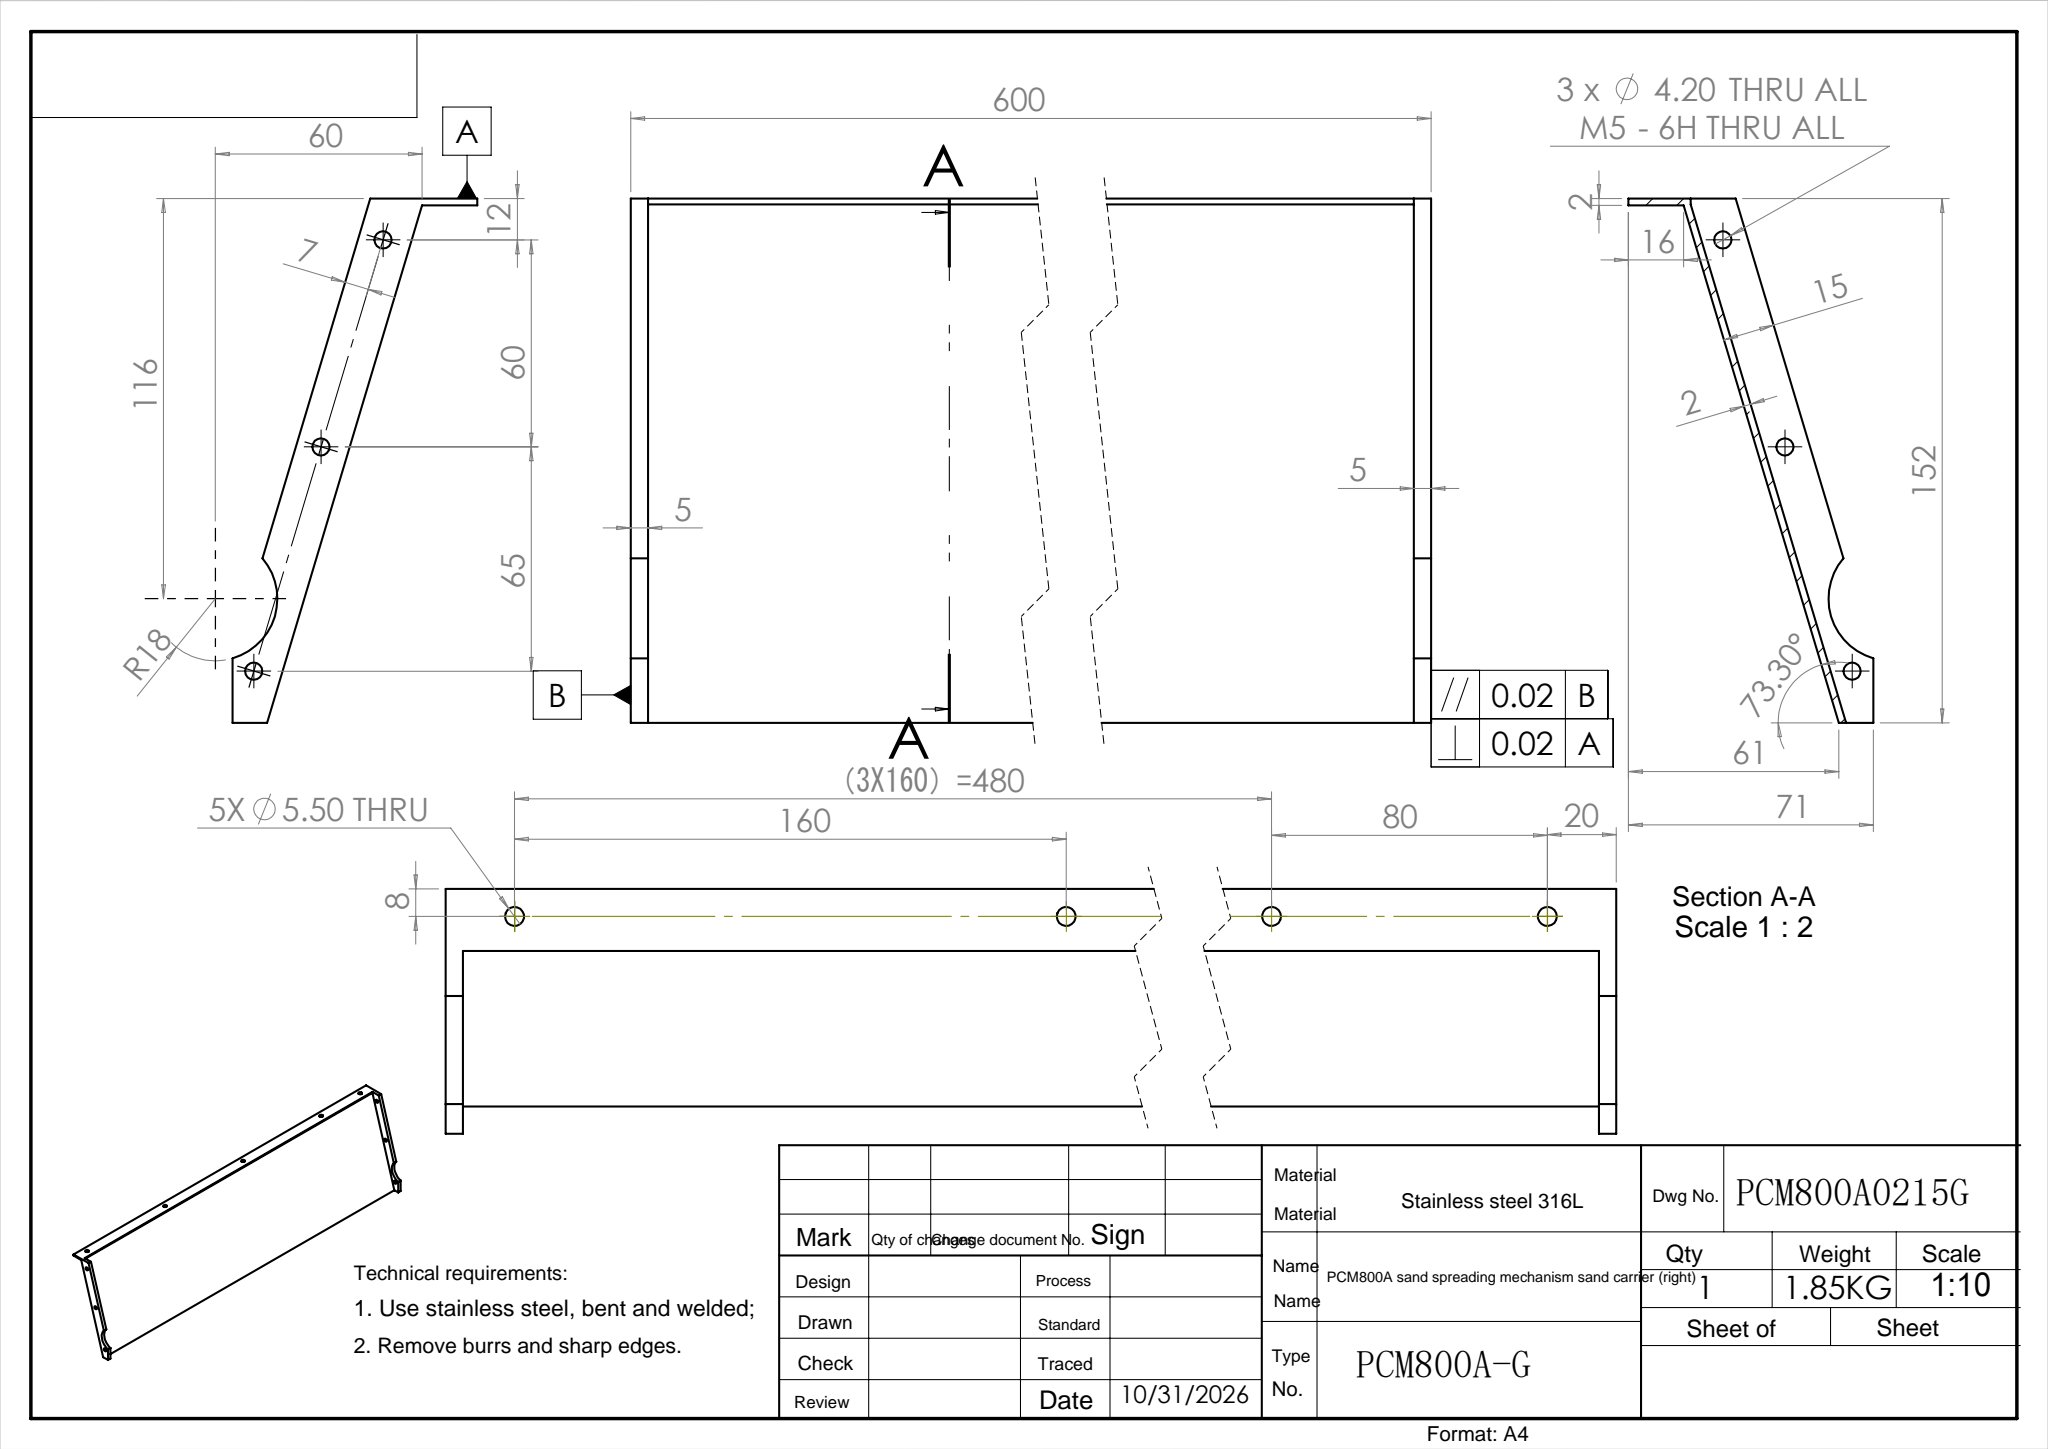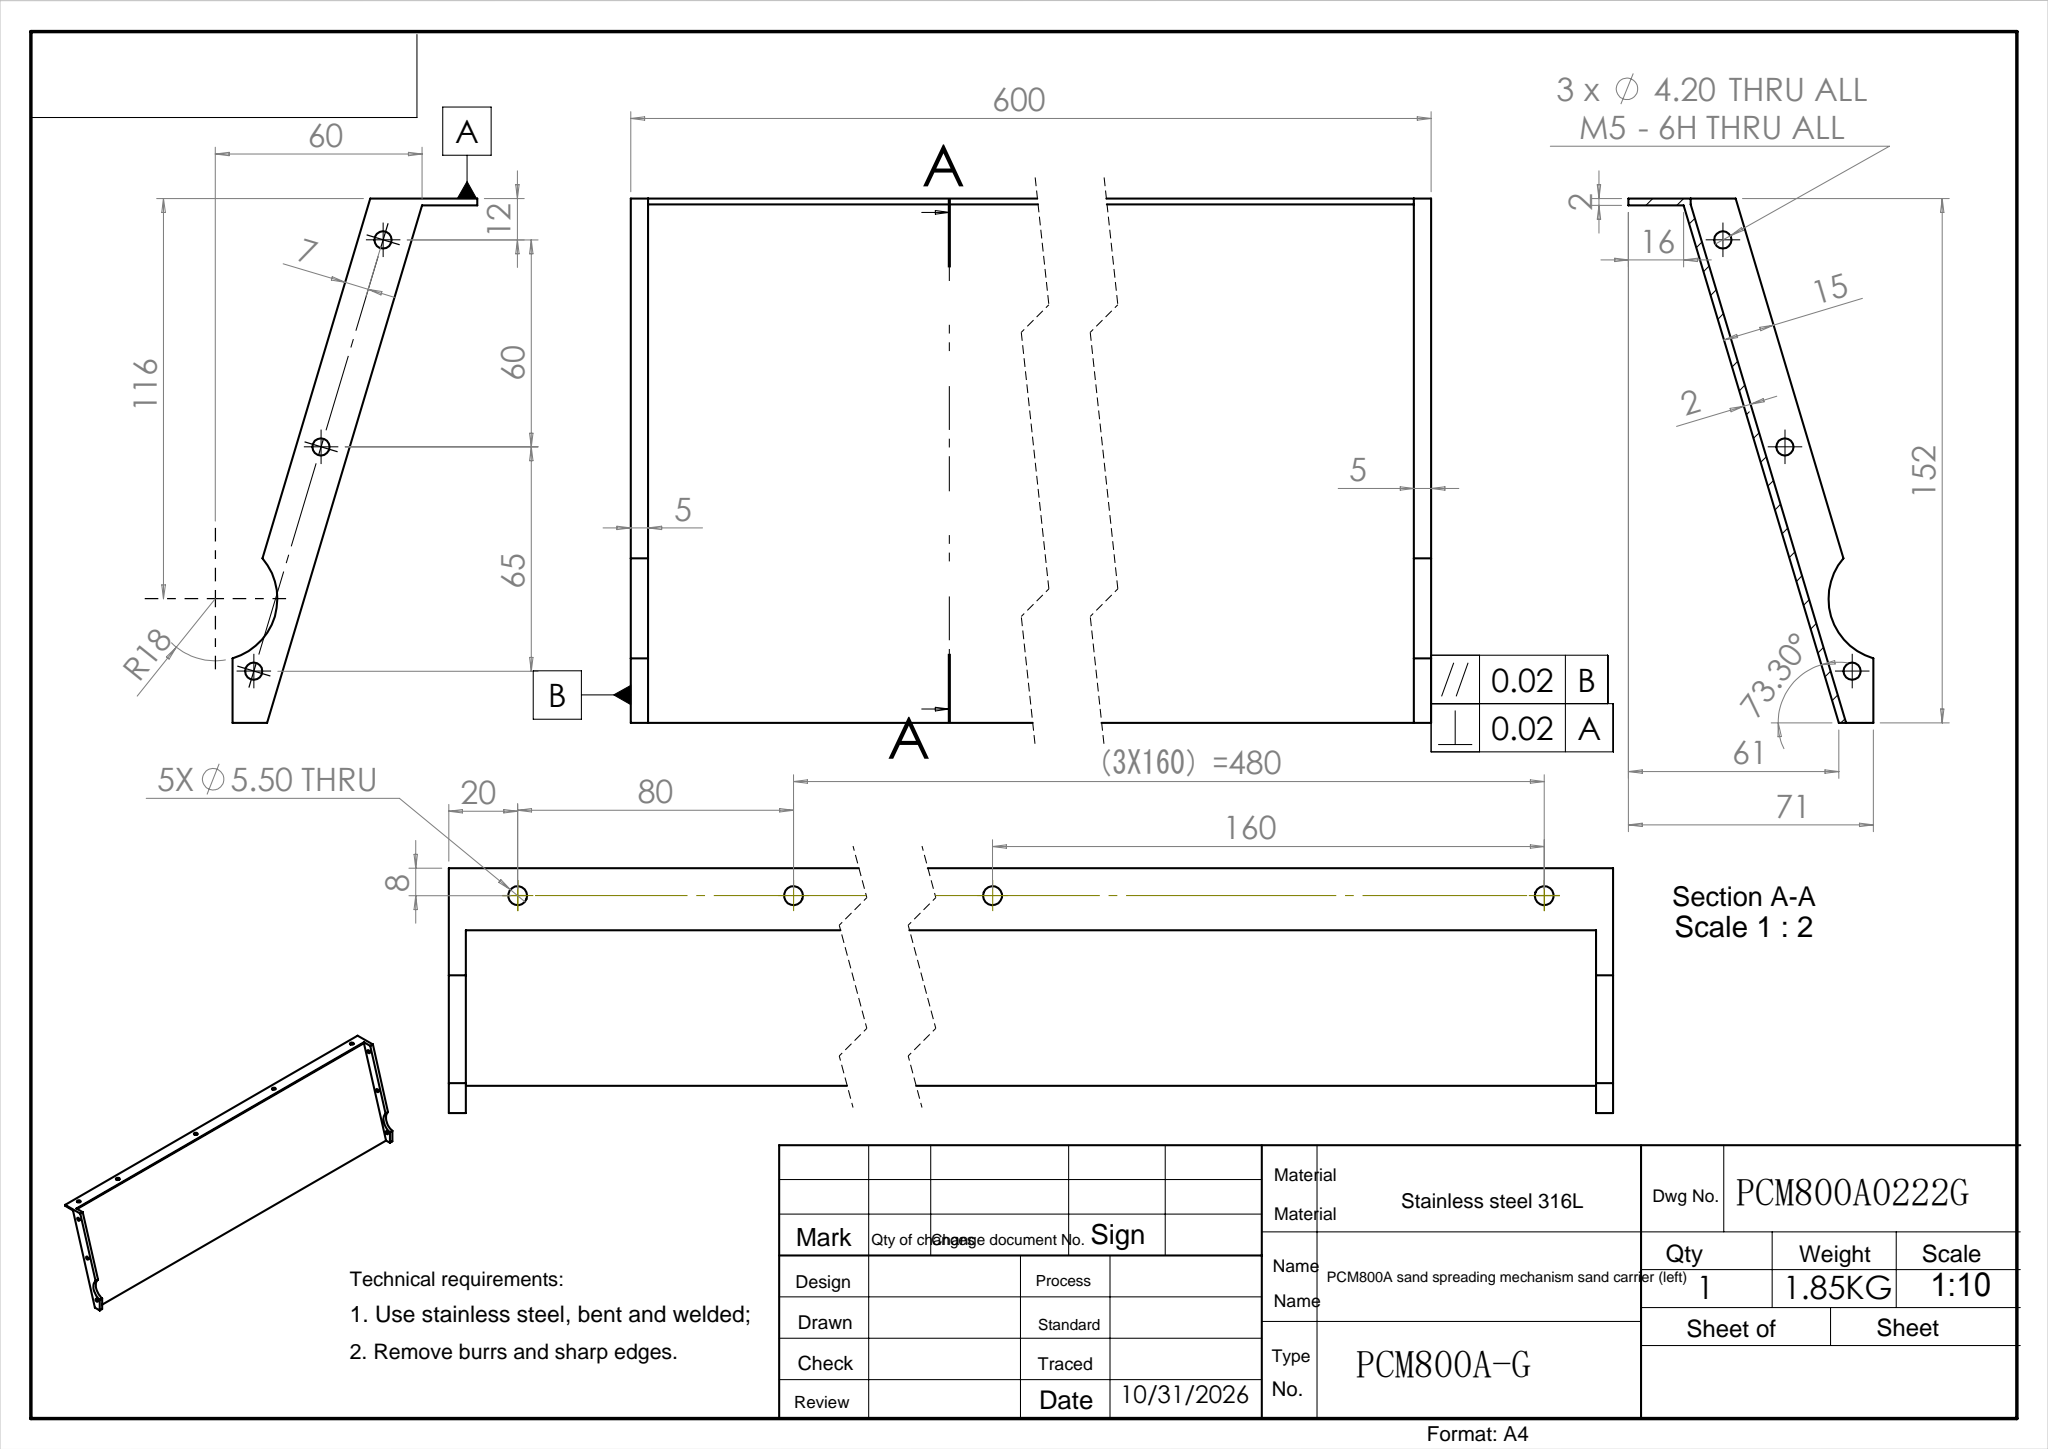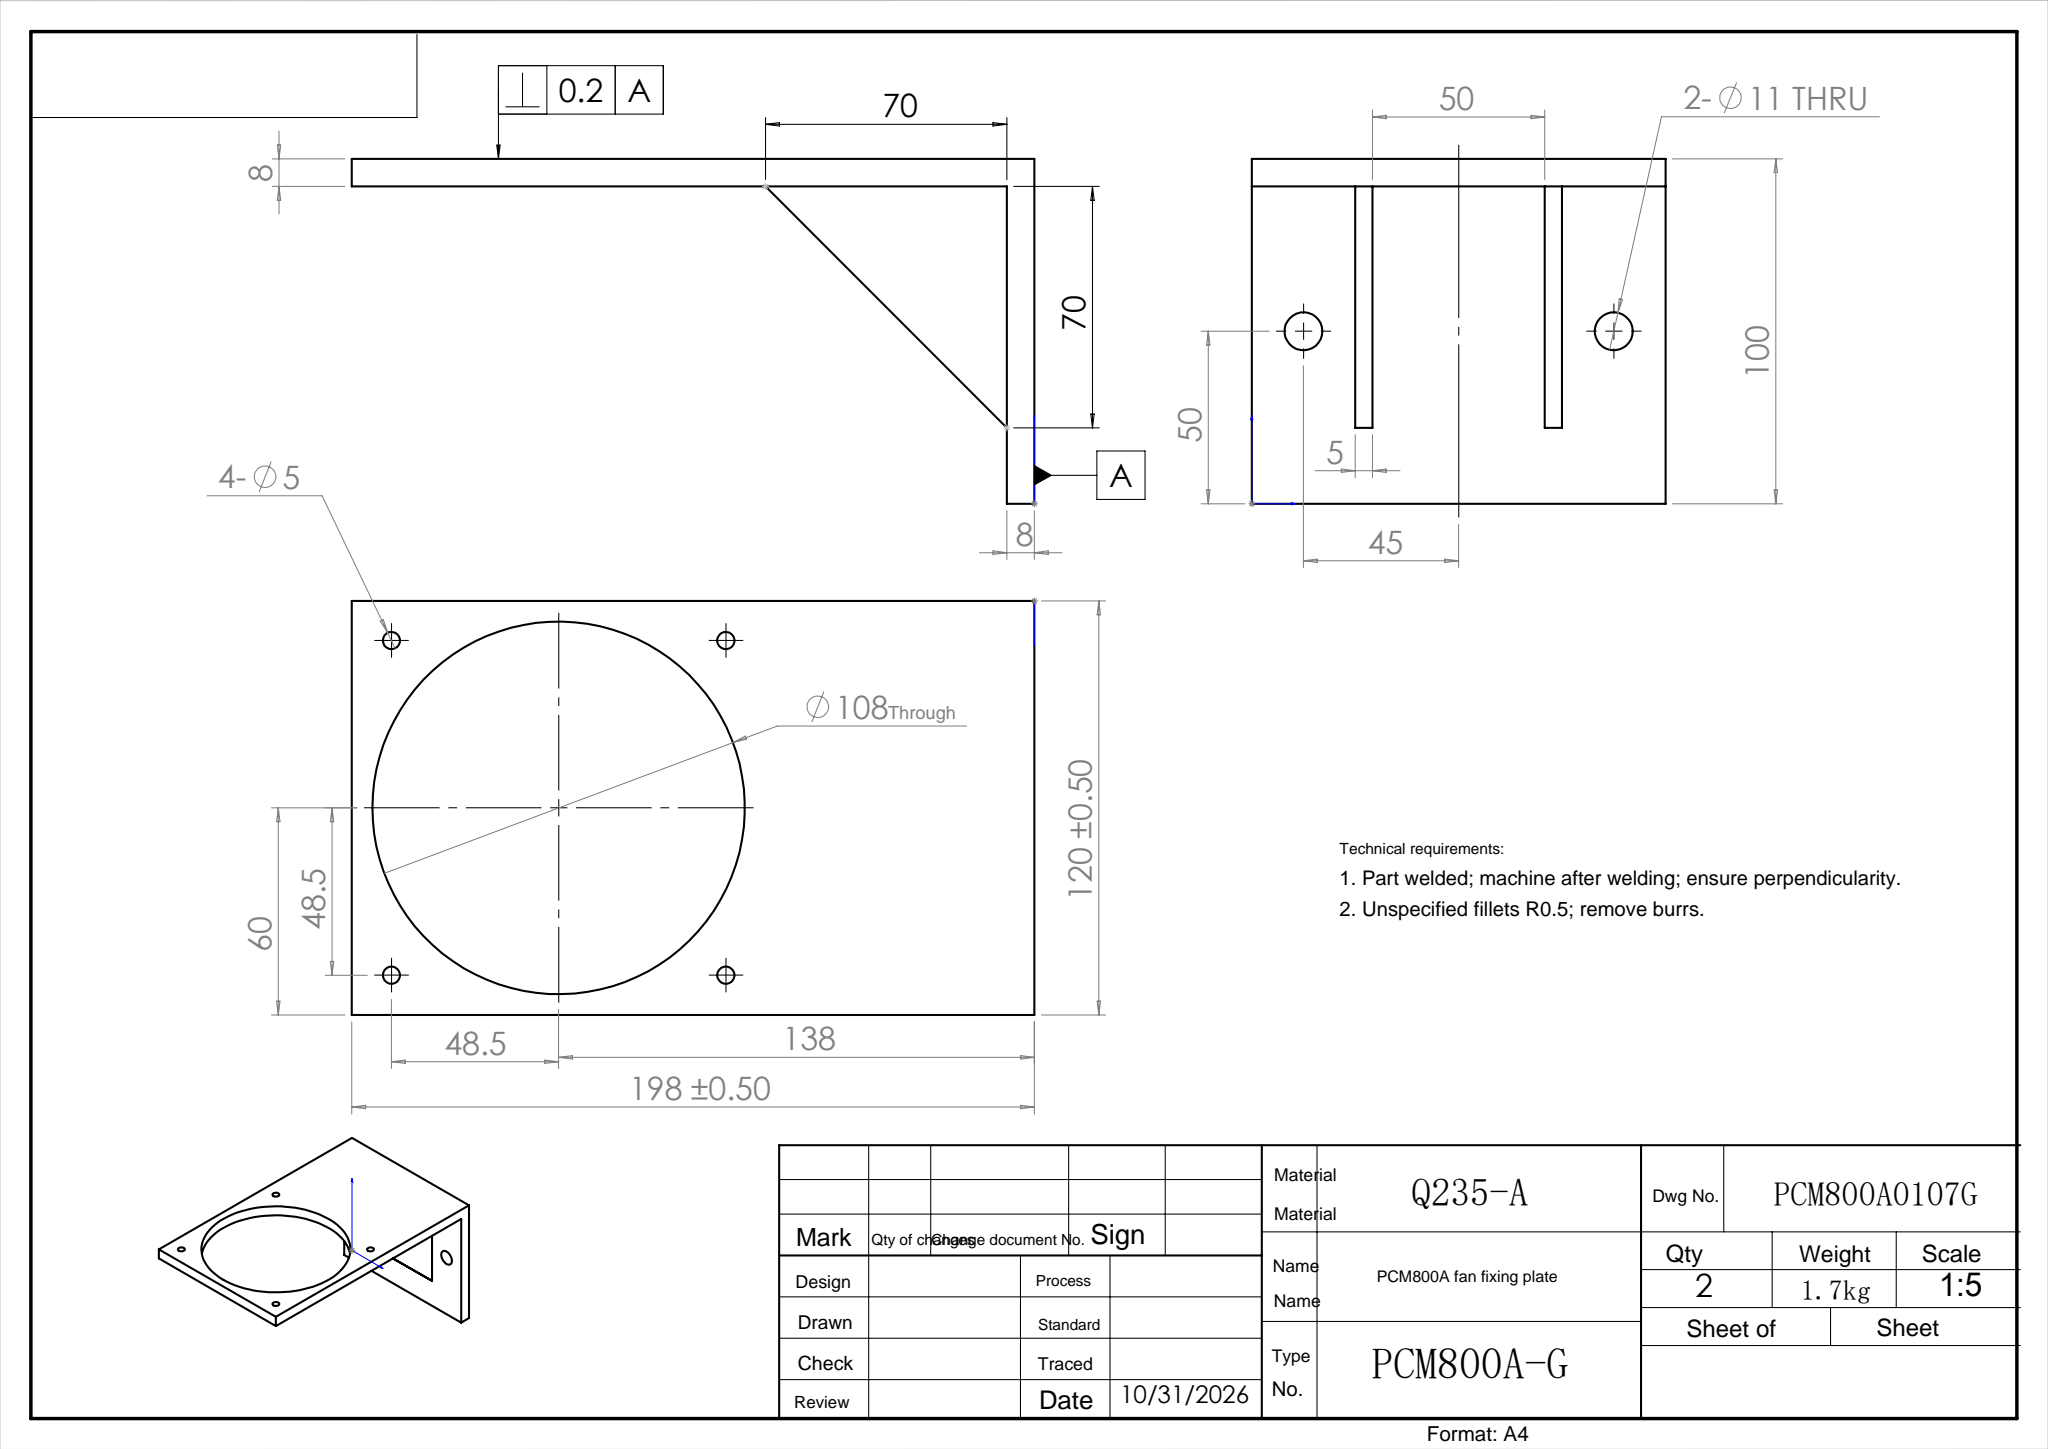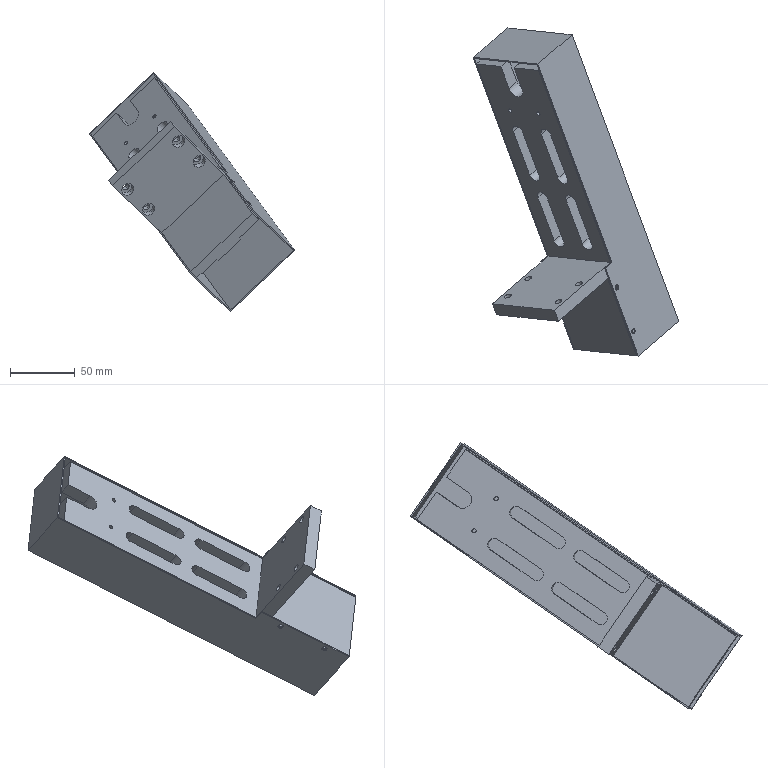Part | SolidWorks | 5 solids | 166 faces | box 158.75 x 253.079 x 184.571 mm | volume 227945 mm3 | plane 77 | cylinder 61 | cone 20 | torus 8 | commonest cylinder face diameters 10 x16 2.5 x8 4 x8 5 x8 5.5 x8 3.3 x4